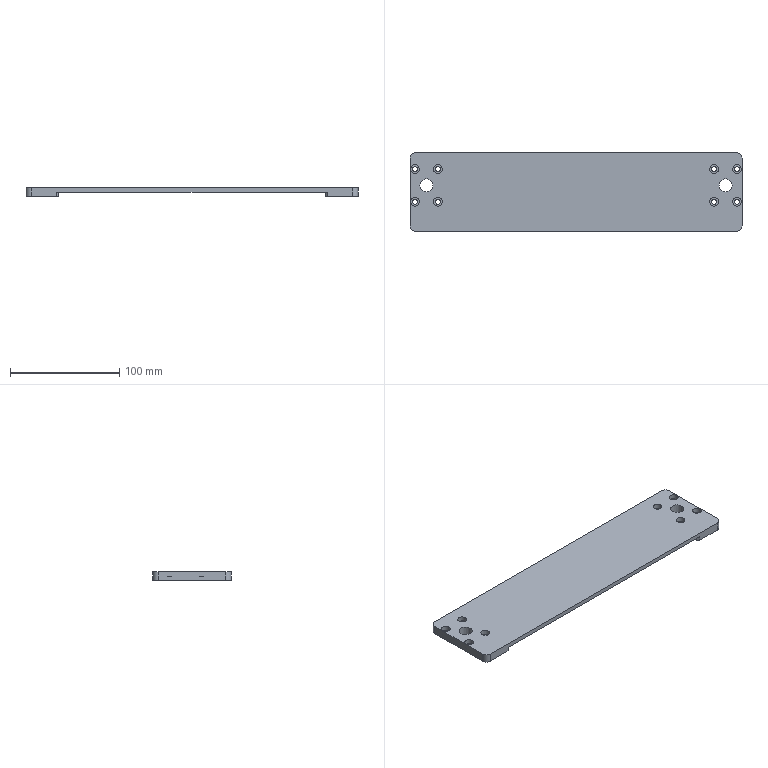CAM job | NX | 3-axis milling, drilling | part box 304 x 72 x 8 mm | stock box 309 x 77 x 10 mm
Tools:
number,name,description,diameter,corner_radius,flute_length,length,flutes
4,D4,平底铣刀-粗,4.0,0.0,25.0,75.0,2
6,D6,平底铣刀-粗,6.0,0.0,25.0,75.0,2
9,D10,平底铣刀-粗,10.0,0.0,35.0,75.0,2
7,D6-J,平底铣刀-精,6.0,0.0,25.0,75.0,2
10,D10-J,平底铣刀-精,10.0,0.0,35.0,75.0,2
1,D80R0.8飞刀,圆鼻刀-粗,80.0,0.8,50.0,75.0,2
1,D80R0.8飞刀-J,圆鼻刀-精,80.0,0.8,50.0,75.0,2
2,D6倒角刀,倒角刀,6.0,0.0,3.0,25.0,2
11,ZT4.5,钻头,4.5,0.0,35.0,50.0,2
17,ZT12,钻头,12.0,0.0,35.0,50.0,2
Operations:
program,operation,operation_type,tool,method,geometry_group,spindle_rpm,surface_speed,feed_per_tooth,feed_cut,feed_plunge,cut_length_mm,path_length_mm,cut_time_min,machine_time_min
B,底壁铣飞面一刀开粗_COPY,VolumeBased25DMillingOperation,D80R0.8飞刀,分层开粗-切深K-步距G,W-B,2800.0,703.696,0.5357,3000.0,100.0,1648.776,2907.734,0.5496,0.6755
B,底壁铣飞面一刀精光_COPY,VolumeBased25DMillingOperation,D80R0.8飞刀-J,侧刃精光-切深K-步距G,W-B,4000.0,1005.28,0.125,1000.0,100.0,411.998,447.998,0.412,0.4156
B,底壁铣分层开粗-中_COPY,VolumeBased25DMillingOperation,D6,分层开粗-切深K-步距G,W-B,6000.0,188.496,0.3333,4000.0,100.0,37992.657,38289.009,9.498,9.528
B,钻倒角_1,Operation,D6倒角刀,METHOD,W-B,8000.0,150.796,0.0625,1000.0,0.0,44.4,547.97,0.0444,0.0948
B,铣倒角_3,PlanarMilling,D6倒角刀,METHOD,W-B,8000.0,150.796,0.075,1200.0,100.0,87.451,443.517,0.0729,0.1085
B,平面去毛刺6X45L_COPY,SurfaceContour,D6倒角刀,爬面_倒角-切深0-步距G,W-B,6500.0,122.519,0.1154,1500.0,100.0,1100.056,2194.035,0.7334,0.8428
B,底壁铣精光底面-中_COPY,VolumeBased25DMillingOperation,D6-J,精光步距切深关,W-B,6000.0,188.496,0.0833,1000.0,100.0,6079.448,6251.089,6.079,6.097
B,底壁铣精光侧面-中-选底面_COPY,VolumeBased25DMillingOperation,D6-J,侧刃精光-切深K-步距G,W-B,6000.0,188.496,0.0833,1000.0,100.0,172.222,447.817,0.1722,0.1998
A,顶面,FaceMilling,D80R0.8飞刀,侧刃精光-切深K-步距G,W-A,4000.0,1005.31,0.125,1000.0,100.0,832.667,868.667,0.8327,0.8363
A,外形粗_2,VolumeBased25DMillingOperation,D10,METHOD,W-A,8000.0,251.327,0.3125,5000.0,80.0,9307.026,9353.626,1.861,1.866
A,沉头孔打点-深0.8,Operation,D6倒角刀,NONE,W-A,8000.0,150.796,0.0312,500.0,90.0,18.0,495.446,0.036,0.0837
A,沉头孔-钻孔0段,Operation,ZT4.5,NONE,W-A,2800.0,39.584,0.0179,100.0,90.0,98.816,641.761,0.9882,1.042
A,通孔-精孔12.0预钻,Operation,ZT12,NONE,W-A,800.0,29.657,0.125,200.0,90.0,28.21,371.423,0.1411,0.1754
A,铣孔开粗D4_1,CylinderMilling,D4,NONE,W-A,8000.0,100.531,0.075,1200.0,100.0,1703.655,2458.474,1.42,1.495
A,铣孔精光D4_1,CylinderMilling,D4,精光步距切深关,W-A,8000.0,100.531,0.0312,500.0,100.0,256.369,1011.188,0.5127,0.5882
A,仅选体,SurfaceContour,D6倒角刀,METHOD,W-A,8000.0,150.796,0.1875,3000.0,100.0,760.731,796.532,0.2536,0.2572
A,铣倒角_1,PlanarMilling,D6倒角刀,NONE,W-A,8000.0,150.796,0.0312,500.0,100.0,271.743,951.818,0.5435,0.6115
A,铣倒角_2,PlanarMilling,D6倒角刀,METHOD,W-A,8000.0,150.796,0.0312,500.0,100.0,87.451,443.517,0.1749,0.2105
A,外形半精_2,VolumeBased25DMillingOperation,D10-J,METHOD,W-A,8000.0,251.327,0.0625,1000.0,100.0,779.828,835.028,0.7798,0.7853